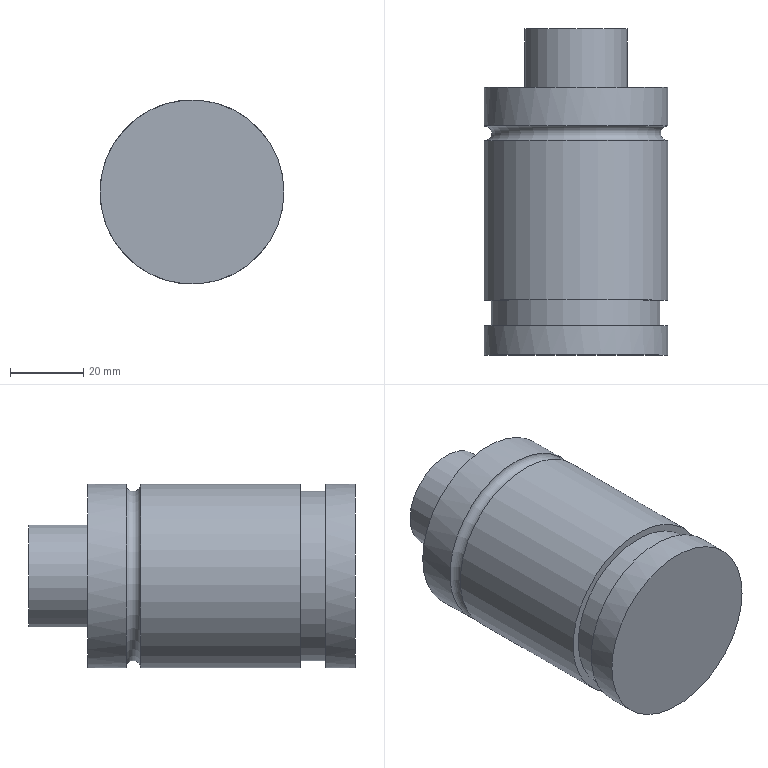Part | NX | features MAIN_BODY 2 | 1 solid | 11 faces | box 50.2 x 89 x 50.2 mm | volume 151259 mm3 | cylinder 5 | plane 5 | torus 1 | commonest cylinder face diameters 50.2 x3 28 x1 46.2 x1
STEP:
#1=CARTESIAN_POINT('',(-999.9,-809.,-395.));
#2=VERTEX_POINT('',#1);
#3=CARTESIAN_POINT('',(-1025.,-809.,-395.));
#4=DIRECTION('',(0.,-1.,0.));
#5=DIRECTION('',(1.,0.,0.));
#6=AXIS2_PLACEMENT_3D('',#3,#4,#5);
#7=CIRCLE('',#6,25.1);
#8=EDGE_CURVE('',#2,#2,#7,.F.);
#9=ORIENTED_EDGE('',*,*,#8,.T.);
#10=EDGE_LOOP('',(#9));
#11=FACE_BOUND('',#10,.T.);
#12=CARTESIAN_POINT('',(-999.9,-765.5,-395.));
#13=VERTEX_POINT('',#12);
#14=CARTESIAN_POINT('',(-1025.,-765.5,-395.));
#15=DIRECTION('',(0.,-1.,0.));
#16=DIRECTION('',(1.,0.,0.));
#17=AXIS2_PLACEMENT_3D('',#14,#15,#16);
#18=CIRCLE('',#17,25.1);
#19=EDGE_CURVE('',#13,#13,#18,.T.);
#20=ORIENTED_EDGE('',*,*,#19,.T.);
#21=EDGE_LOOP('',(#20));
#22=FACE_BOUND('',#21,.T.);
#23=CARTESIAN_POINT('',(-1025.,-751.,-395.));
#24=DIRECTION('',(0.,-1.,0.));
#25=DIRECTION('',(1.,0.,0.));
#26=AXIS2_PLACEMENT_3D('',#23,#24,#25);
#27=CYLINDRICAL_SURFACE('',#26,25.1);
#28=ADVANCED_FACE('',(#11,#22),#27,.T.);
#29=CARTESIAN_POINT('',(-1050.1,-751.,-395.));
#30=VERTEX_POINT('',#29);
#31=CARTESIAN_POINT('',(-1025.,-751.,-395.));
#32=DIRECTION('',(0.,1.,0.));
#33=DIRECTION('',(-1.,0.,0.));
#34=AXIS2_PLACEMENT_3D('',#31,#32,#33);
#35=CIRCLE('',#34,25.1);
#36=EDGE_CURVE('',#30,#30,#35,.T.);
#37=ORIENTED_EDGE('',*,*,#36,.T.);
#38=EDGE_LOOP('',(#37));
#39=FACE_BOUND('',#38,.T.);
#40=CARTESIAN_POINT('',(-1039.,-751.,-395.));
#41=VERTEX_POINT('',#40);
#42=CARTESIAN_POINT('',(-1025.,-751.,-395.));
#43=DIRECTION('',(0.,1.,0.));
#44=DIRECTION('',(-1.,0.,0.));
#45=AXIS2_PLACEMENT_3D('',#42,#43,#44);
#46=CIRCLE('',#45,14.);
#47=EDGE_CURVE('',#41,#41,#46,.T.);
#48=ORIENTED_EDGE('',*,*,#47,.F.);
#49=EDGE_LOOP('',(#48));
#50=FACE_BOUND('',#49,.T.);
#51=CARTESIAN_POINT('',(-1025.,-751.,-395.));
#52=DIRECTION('',(0.,1.,0.));
#53=DIRECTION('',(-1.,0.,0.));
#54=AXIS2_PLACEMENT_3D('',#51,#52,#53);
#55=PLANE('',#54);
#56=ADVANCED_FACE('',(#39,#50),#55,.T.);
#57=CARTESIAN_POINT('',(-999.9,-761.5,-395.));
#58=VERTEX_POINT('',#57);
#59=CARTESIAN_POINT('',(-1025.,-761.5,-395.));
#60=DIRECTION('',(0.,-1.,0.));
#61=DIRECTION('',(1.,0.,0.));
#62=AXIS2_PLACEMENT_3D('',#59,#60,#61);
#63=CIRCLE('',#62,25.1);
#64=EDGE_CURVE('',#58,#58,#63,.F.);
#65=ORIENTED_EDGE('',*,*,#64,.T.);
#66=EDGE_LOOP('',(#65));
#67=FACE_BOUND('',#66,.T.);
#68=ORIENTED_EDGE('',*,*,#36,.F.);
#69=EDGE_LOOP('',(#68));
#70=FACE_BOUND('',#69,.T.);
#71=CARTESIAN_POINT('',(-1025.,-751.,-395.));
#72=DIRECTION('',(0.,-1.,0.));
#73=DIRECTION('',(1.,0.,0.));
#74=AXIS2_PLACEMENT_3D('',#71,#72,#73);
#75=CYLINDRICAL_SURFACE('',#74,25.1);
#76=ADVANCED_FACE('',(#67,#70),#75,.T.);
#77=CARTESIAN_POINT('',(-1039.,-735.,-395.));
#78=VERTEX_POINT('',#77);
#79=CARTESIAN_POINT('',(-1025.,-735.,-395.));
#80=DIRECTION('',(0.,1.,0.));
#81=DIRECTION('',(-1.,0.,0.));
#82=AXIS2_PLACEMENT_3D('',#79,#80,#81);
#83=CIRCLE('',#82,14.);
#84=EDGE_CURVE('',#78,#78,#83,.T.);
#85=ORIENTED_EDGE('',*,*,#84,.F.);
#86=EDGE_LOOP('',(#85));
#87=FACE_BOUND('',#86,.T.);
#88=ORIENTED_EDGE('',*,*,#47,.T.);
#89=EDGE_LOOP('',(#88));
#90=FACE_BOUND('',#89,.T.);
#91=CARTESIAN_POINT('',(-1025.,-748.,-395.));
#92=DIRECTION('',(0.,-1.,0.));
#93=DIRECTION('',(1.,0.,0.));
#94=AXIS2_PLACEMENT_3D('',#91,#92,#93);
#95=CYLINDRICAL_SURFACE('',#94,14.);
#96=ADVANCED_FACE('',(#87,#90),#95,.T.);
#97=ORIENTED_EDGE('',*,*,#64,.F.);
#98=EDGE_LOOP('',(#97));
#99=FACE_BOUND('',#98,.T.);
#100=ORIENTED_EDGE('',*,*,#19,.F.);
#101=EDGE_LOOP('',(#100));
#102=FACE_BOUND('',#101,.T.);
#103=CARTESIAN_POINT('',(-1025.,-763.5,-395.));
#104=DIRECTION('',(0.,-1.,0.));
#105=DIRECTION('',(1.,0.,0.));
#106=AXIS2_PLACEMENT_3D('',#103,#104,#105);
#107=TOROIDAL_SURFACE('',#106,25.1,2.);
#108=ADVANCED_FACE('',(#99,#102),#107,.F.);
#109=CARTESIAN_POINT('',(-1048.1,-809.,-395.));
#110=VERTEX_POINT('',#109);
#111=CARTESIAN_POINT('',(-1025.,-809.,-395.));
#112=DIRECTION('',(0.,1.,0.));
#113=DIRECTION('',(-1.,0.,0.));
#114=AXIS2_PLACEMENT_3D('',#111,#112,#113);
#115=CIRCLE('',#114,23.1);
#116=EDGE_CURVE('',#110,#110,#115,.T.);
#117=ORIENTED_EDGE('',*,*,#116,.T.);
#118=EDGE_LOOP('',(#117));
#119=FACE_BOUND('',#118,.T.);
#120=ORIENTED_EDGE('',*,*,#8,.F.);
#121=EDGE_LOOP('',(#120));
#122=FACE_BOUND('',#121,.T.);
#123=CARTESIAN_POINT('',(-1025.,-809.,-395.));
#124=DIRECTION('',(0.,-1.,0.));
#125=DIRECTION('',(1.,0.,0.));
#126=AXIS2_PLACEMENT_3D('',#123,#124,#125);
#127=PLANE('',#126);
#128=ADVANCED_FACE('',(#119,#122),#127,.T.);
#129=CARTESIAN_POINT('',(-1048.1,-816.,-395.));
#130=VERTEX_POINT('',#129);
#131=CARTESIAN_POINT('',(-1025.,-816.,-395.));
#132=DIRECTION('',(0.,1.,0.));
#133=DIRECTION('',(-1.,0.,0.));
#134=AXIS2_PLACEMENT_3D('',#131,#132,#133);
#135=CIRCLE('',#134,23.1);
#136=EDGE_CURVE('',#130,#130,#135,.T.);
#137=ORIENTED_EDGE('',*,*,#136,.F.);
#138=EDGE_LOOP('',(#137));
#139=FACE_BOUND('',#138,.T.);
#140=CARTESIAN_POINT('',(-999.9,-816.,-395.));
#141=VERTEX_POINT('',#140);
#142=CARTESIAN_POINT('',(-1025.,-816.,-395.));
#143=DIRECTION('',(0.,-1.,0.));
#144=DIRECTION('',(1.,0.,0.));
#145=AXIS2_PLACEMENT_3D('',#142,#143,#144);
#146=CIRCLE('',#145,25.1);
#147=EDGE_CURVE('',#141,#141,#146,.T.);
#148=ORIENTED_EDGE('',*,*,#147,.F.);
#149=EDGE_LOOP('',(#148));
#150=FACE_BOUND('',#149,.T.);
#151=CARTESIAN_POINT('',(-1025.,-816.,-395.));
#152=DIRECTION('',(0.,-1.,0.));
#153=DIRECTION('',(1.,0.,0.));
#154=AXIS2_PLACEMENT_3D('',#151,#152,#153);
#155=PLANE('',#154);
#156=ADVANCED_FACE('',(#139,#150),#155,.F.);
#157=ORIENTED_EDGE('',*,*,#116,.F.);
#158=EDGE_LOOP('',(#157));
#159=FACE_BOUND('',#158,.T.);
#160=ORIENTED_EDGE('',*,*,#136,.T.);
#161=EDGE_LOOP('',(#160));
#162=FACE_BOUND('',#161,.T.);
#163=CARTESIAN_POINT('',(-1025.,-816.,-395.));
#164=DIRECTION('',(0.,1.,0.));
#165=DIRECTION('',(-1.,0.,0.));
#166=AXIS2_PLACEMENT_3D('',#163,#164,#165);
#167=CYLINDRICAL_SURFACE('',#166,23.1);
#168=ADVANCED_FACE('',(#159,#162),#167,.T.);
#169=CARTESIAN_POINT('',(-1050.1,-824.,-395.));
#170=VERTEX_POINT('',#169);
#171=CARTESIAN_POINT('',(-1025.,-824.,-395.));
#172=DIRECTION('',(0.,1.,0.));
#173=DIRECTION('',(-1.,0.,0.));
#174=AXIS2_PLACEMENT_3D('',#171,#172,#173);
#175=CIRCLE('',#174,25.1);
#176=EDGE_CURVE('',#170,#170,#175,.T.);
#177=ORIENTED_EDGE('',*,*,#176,.F.);
#178=EDGE_LOOP('',(#177));
#179=FACE_BOUND('',#178,.T.);
#180=CARTESIAN_POINT('',(-1025.,-824.,-395.));
#181=DIRECTION('',(0.,1.,0.));
#182=DIRECTION('',(-1.,0.,0.));
#183=AXIS2_PLACEMENT_3D('',#180,#181,#182);
#184=PLANE('',#183);
#185=ADVANCED_FACE('',(#179),#184,.F.);
#186=ORIENTED_EDGE('',*,*,#147,.T.);
#187=EDGE_LOOP('',(#186));
#188=FACE_BOUND('',#187,.T.);
#189=ORIENTED_EDGE('',*,*,#176,.T.);
#190=EDGE_LOOP('',(#189));
#191=FACE_BOUND('',#190,.T.);
#192=CARTESIAN_POINT('',(-1025.,-751.,-395.));
#193=DIRECTION('',(0.,-1.,0.));
#194=DIRECTION('',(1.,0.,0.));
#195=AXIS2_PLACEMENT_3D('',#192,#193,#194);
#196=CYLINDRICAL_SURFACE('',#195,25.1);
#197=ADVANCED_FACE('',(#188,#191),#196,.T.);
#198=ORIENTED_EDGE('',*,*,#84,.T.);
#199=EDGE_LOOP('',(#198));
#200=FACE_BOUND('',#199,.T.);
#201=CARTESIAN_POINT('',(-1025.,-735.,-395.));
#202=DIRECTION('',(0.,1.,0.));
#203=DIRECTION('',(-1.,0.,0.));
#204=AXIS2_PLACEMENT_3D('',#201,#202,#203);
#205=PLANE('',#204);
#206=ADVANCED_FACE('',(#200),#205,.T.);
#207=CLOSED_SHELL('',(#28,#56,#76,#96,#108,#128,#156,#168,#185,#197,#206));
#208=MANIFOLD_SOLID_BREP('',#207);
#209=(LENGTH_UNIT()NAMED_UNIT(*)SI_UNIT(.MILLI.,.METRE.));
#210=UNCERTAINTY_MEASURE_WITH_UNIT(LENGTH_MEASURE(0.00001),#209,'','');
#211=(NAMED_UNIT(*)PLANE_ANGLE_UNIT()SI_UNIT($,.RADIAN.));
#212=(NAMED_UNIT(*)SI_UNIT($,.STERADIAN.)SOLID_ANGLE_UNIT());
#213=(GEOMETRIC_REPRESENTATION_CONTEXT(3)GLOBAL_UNCERTAINTY_ASSIGNED_CONTEXT((#210))GLOBAL_UNIT_ASSIGNED_CONTEXT((#209,#211,#212))REPRESENTATION_CONTEXT('',''));
#214=ADVANCED_BREP_SHAPE_REPRESENTATION('',(#208),#213);